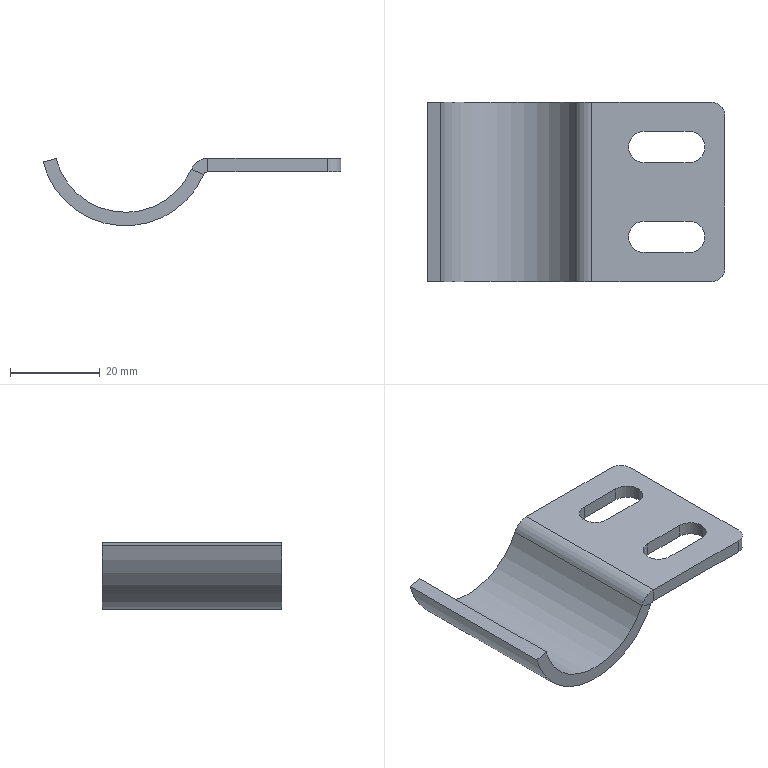Part | STEP file | PN_0001 guardrail connecting plate 1_Default<As Machined> | 1 solid | 24 faces | box 66.397 x 40 x 15 mm | volume 8448 mm3 | plane 14 | cylinder 10 | commonest cylinder face diameters 7 x4 6 x2 2 x1 8 x1 32 x1 38 x1